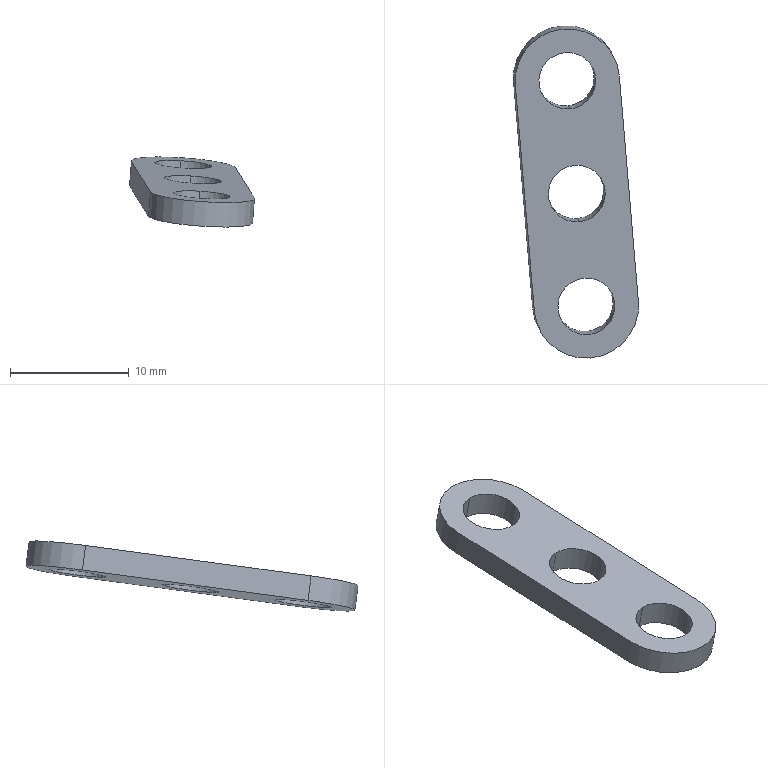Part | SolidWorks | features SplitBody 1 | 1 solid | 13 faces | box 10.521 x 27.955 x 5.897 mm | volume 365.029 mm3 | cylinder 9 | plane 4 | commonest cylinder face diameters 4.8 x6 8.8 x3
STEP:
#1=CARTESIAN_POINT('',(578.818,319.832,-356.747));
#2=VERTEX_POINT('',#1);
#3=CARTESIAN_POINT('',(579.217,315.091,-357.386));
#4=VERTEX_POINT('',#3);
#5=CARTESIAN_POINT('',(579.017,317.461,-357.067));
#6=DIRECTION('',(-0.07028,0.1275,-0.9893));
#7=DIRECTION('',(0.08315,-0.9876,-0.1332));
#8=AXIS2_PLACEMENT_3D('',#5,#6,#7);
#9=CIRCLE('',#8,2.4);
#10=EDGE_CURVE('',#2,#4,#9,.T.);
#11=ORIENTED_EDGE('',*,*,#10,.T.);
#12=CARTESIAN_POINT('',(579.363,314.826,-355.329));
#13=VERTEX_POINT('',#12);
#14=CARTESIAN_POINT('',(579.217,315.091,-357.386));
#15=DIRECTION('',(0.07028,-0.1275,0.9893));
#16=VECTOR('',#15,1000.);
#17=LINE('',#14,#16);
#18=EDGE_CURVE('',#4,#13,#17,.T.);
#19=ORIENTED_EDGE('',*,*,#18,.T.);
#20=CARTESIAN_POINT('',(578.964,319.566,-354.689));
#21=VERTEX_POINT('',#20);
#22=CARTESIAN_POINT('',(579.163,317.196,-355.009));
#23=DIRECTION('',(-0.07028,0.1275,-0.9893));
#24=DIRECTION('',(0.08315,-0.9876,-0.1332));
#25=AXIS2_PLACEMENT_3D('',#22,#23,#24);
#26=CIRCLE('',#25,2.4);
#27=EDGE_CURVE('',#21,#13,#26,.T.);
#28=ORIENTED_EDGE('',*,*,#27,.F.);
#29=CARTESIAN_POINT('',(578.818,319.832,-356.747));
#30=DIRECTION('',(0.07028,-0.1275,0.9893));
#31=VECTOR('',#30,1000.);
#32=LINE('',#29,#31);
#33=EDGE_CURVE('',#2,#21,#32,.T.);
#34=ORIENTED_EDGE('',*,*,#33,.F.);
#35=EDGE_LOOP('',(#11,#19,#28,#34));
#36=FACE_OUTER_BOUND('',#35,.T.);
#37=CARTESIAN_POINT('',(579.017,317.461,-357.067));
#38=DIRECTION('',(0.07028,-0.1275,0.9893));
#39=DIRECTION('',(-0.08315,0.9876,0.1332));
#40=AXIS2_PLACEMENT_3D('',#37,#38,#39);
#41=CYLINDRICAL_SURFACE('',#40,2.4);
#42=ADVANCED_FACE('',(#36),#41,.F.);
#43=CARTESIAN_POINT('',(578.019,329.312,-355.468));
#44=VERTEX_POINT('',#43);
#45=CARTESIAN_POINT('',(578.418,324.572,-356.108));
#46=VERTEX_POINT('',#45);
#47=CARTESIAN_POINT('',(578.219,326.942,-355.788));
#48=DIRECTION('',(-0.07028,0.1275,-0.9893));
#49=DIRECTION('',(0.08315,-0.9876,-0.1332));
#50=AXIS2_PLACEMENT_3D('',#47,#48,#49);
#51=CIRCLE('',#50,2.4);
#52=EDGE_CURVE('',#44,#46,#51,.T.);
#53=ORIENTED_EDGE('',*,*,#52,.T.);
#54=CARTESIAN_POINT('',(578.565,324.307,-354.05));
#55=VERTEX_POINT('',#54);
#56=CARTESIAN_POINT('',(578.418,324.572,-356.108));
#57=DIRECTION('',(0.07028,-0.1275,0.9893));
#58=VECTOR('',#57,1000.);
#59=LINE('',#56,#58);
#60=EDGE_CURVE('',#46,#55,#59,.T.);
#61=ORIENTED_EDGE('',*,*,#60,.T.);
#62=CARTESIAN_POINT('',(578.166,329.047,-353.411));
#63=VERTEX_POINT('',#62);
#64=CARTESIAN_POINT('',(578.365,326.677,-353.73));
#65=DIRECTION('',(-0.07028,0.1275,-0.9893));
#66=DIRECTION('',(0.08315,-0.9876,-0.1332));
#67=AXIS2_PLACEMENT_3D('',#64,#65,#66);
#68=CIRCLE('',#67,2.4);
#69=EDGE_CURVE('',#63,#55,#68,.T.);
#70=ORIENTED_EDGE('',*,*,#69,.F.);
#71=CARTESIAN_POINT('',(578.019,329.312,-355.468));
#72=DIRECTION('',(0.07028,-0.1275,0.9893));
#73=VECTOR('',#72,1000.);
#74=LINE('',#71,#73);
#75=EDGE_CURVE('',#44,#63,#74,.T.);
#76=ORIENTED_EDGE('',*,*,#75,.F.);
#77=EDGE_LOOP('',(#53,#61,#70,#76));
#78=FACE_OUTER_BOUND('',#77,.T.);
#79=CARTESIAN_POINT('',(578.219,326.942,-355.788));
#80=DIRECTION('',(0.07028,-0.1275,0.9893));
#81=DIRECTION('',(-0.08315,0.9876,0.1332));
#82=AXIS2_PLACEMENT_3D('',#79,#80,#81);
#83=CYLINDRICAL_SURFACE('',#82,2.4);
#84=ADVANCED_FACE('',(#78),#83,.F.);
#85=CARTESIAN_POINT('',(579.616,310.351,-358.026));
#86=VERTEX_POINT('',#85);
#87=CARTESIAN_POINT('',(580.015,305.61,-358.665));
#88=VERTEX_POINT('',#87);
#89=CARTESIAN_POINT('',(579.815,307.98,-358.345));
#90=DIRECTION('',(-0.07028,0.1275,-0.9893));
#91=DIRECTION('',(0.08315,-0.9876,-0.1332));
#92=AXIS2_PLACEMENT_3D('',#89,#90,#91);
#93=CIRCLE('',#92,2.4);
#94=EDGE_CURVE('',#86,#88,#93,.T.);
#95=ORIENTED_EDGE('',*,*,#94,.T.);
#96=CARTESIAN_POINT('',(580.161,305.345,-356.607));
#97=VERTEX_POINT('',#96);
#98=CARTESIAN_POINT('',(580.015,305.61,-358.665));
#99=DIRECTION('',(0.07028,-0.1275,0.9893));
#100=VECTOR('',#99,1000.);
#101=LINE('',#98,#100);
#102=EDGE_CURVE('',#88,#97,#101,.T.);
#103=ORIENTED_EDGE('',*,*,#102,.T.);
#104=CARTESIAN_POINT('',(579.762,310.085,-355.968));
#105=VERTEX_POINT('',#104);
#106=CARTESIAN_POINT('',(579.962,307.715,-356.288));
#107=DIRECTION('',(-0.07028,0.1275,-0.9893));
#108=DIRECTION('',(0.08315,-0.9876,-0.1332));
#109=AXIS2_PLACEMENT_3D('',#106,#107,#108);
#110=CIRCLE('',#109,2.4);
#111=EDGE_CURVE('',#105,#97,#110,.T.);
#112=ORIENTED_EDGE('',*,*,#111,.F.);
#113=CARTESIAN_POINT('',(579.616,310.351,-358.026));
#114=DIRECTION('',(0.07028,-0.1275,0.9893));
#115=VECTOR('',#114,1000.);
#116=LINE('',#113,#115);
#117=EDGE_CURVE('',#86,#105,#116,.T.);
#118=ORIENTED_EDGE('',*,*,#117,.F.);
#119=EDGE_LOOP('',(#95,#103,#112,#118));
#120=FACE_OUTER_BOUND('',#119,.T.);
#121=CARTESIAN_POINT('',(579.815,307.98,-358.345));
#122=DIRECTION('',(0.07028,-0.1275,0.9893));
#123=DIRECTION('',(-0.08315,0.9876,0.1332));
#124=AXIS2_PLACEMENT_3D('',#121,#122,#123);
#125=CYLINDRICAL_SURFACE('',#124,2.4);
#126=ADVANCED_FACE('',(#120),#125,.F.);
#127=CARTESIAN_POINT('',(577.853,331.288,-355.202));
#128=VERTEX_POINT('',#127);
#129=CARTESIAN_POINT('',(582.593,327.345,-356.047));
#130=VERTEX_POINT('',#129);
#131=CARTESIAN_POINT('',(578.219,326.942,-355.788));
#132=DIRECTION('',(-0.07028,0.1275,-0.9893));
#133=DIRECTION('',(-0.08315,0.9876,0.1332));
#134=AXIS2_PLACEMENT_3D('',#131,#132,#133);
#135=CIRCLE('',#134,4.4);
#136=EDGE_CURVE('',#128,#130,#135,.T.);
#137=ORIENTED_EDGE('',*,*,#136,.F.);
#138=CARTESIAN_POINT('',(577.999,331.022,-353.144));
#139=VERTEX_POINT('',#138);
#140=CARTESIAN_POINT('',(577.853,331.288,-355.202));
#141=DIRECTION('',(0.07028,-0.1275,0.9893));
#142=VECTOR('',#141,1000.);
#143=LINE('',#140,#142);
#144=EDGE_CURVE('',#128,#139,#143,.T.);
#145=ORIENTED_EDGE('',*,*,#144,.T.);
#146=CARTESIAN_POINT('',(582.739,327.08,-353.989));
#147=VERTEX_POINT('',#146);
#148=CARTESIAN_POINT('',(578.365,326.677,-353.73));
#149=DIRECTION('',(-0.07028,0.1275,-0.9893));
#150=DIRECTION('',(-0.08315,0.9876,0.1332));
#151=AXIS2_PLACEMENT_3D('',#148,#149,#150);
#152=CIRCLE('',#151,4.4);
#153=EDGE_CURVE('',#139,#147,#152,.T.);
#154=ORIENTED_EDGE('',*,*,#153,.T.);
#155=CARTESIAN_POINT('',(582.593,327.345,-356.047));
#156=DIRECTION('',(0.07028,-0.1275,0.9893));
#157=VECTOR('',#156,1000.);
#158=LINE('',#155,#157);
#159=EDGE_CURVE('',#130,#147,#158,.T.);
#160=ORIENTED_EDGE('',*,*,#159,.F.);
#161=EDGE_LOOP('',(#137,#145,#154,#160));
#162=FACE_OUTER_BOUND('',#161,.T.);
#163=CARTESIAN_POINT('',(578.219,326.942,-355.788));
#164=DIRECTION('',(0.07028,-0.1275,0.9893));
#165=DIRECTION('',(-0.08315,0.9876,0.1332));
#166=AXIS2_PLACEMENT_3D('',#163,#164,#165);
#167=CYLINDRICAL_SURFACE('',#166,4.4);
#168=ADVANCED_FACE('',(#162),#167,.T.);
#169=CARTESIAN_POINT('',(573.845,326.539,-355.529));
#170=VERTEX_POINT('',#169);
#171=CARTESIAN_POINT('',(578.219,326.942,-355.788));
#172=DIRECTION('',(-0.07028,0.1275,-0.9893));
#173=DIRECTION('',(-0.08315,0.9876,0.1332));
#174=AXIS2_PLACEMENT_3D('',#171,#172,#173);
#175=CIRCLE('',#174,4.4);
#176=EDGE_CURVE('',#170,#128,#175,.T.);
#177=ORIENTED_EDGE('',*,*,#176,.T.);
#178=ORIENTED_EDGE('',*,*,#136,.T.);
#179=CARTESIAN_POINT('',(584.189,308.384,-358.604));
#180=VERTEX_POINT('',#179);
#181=CARTESIAN_POINT('',(582.593,327.345,-356.047));
#182=DIRECTION('',(0.08315,-0.9876,-0.1332));
#183=VECTOR('',#182,1000.);
#184=LINE('',#181,#183);
#185=EDGE_CURVE('',#130,#180,#184,.T.);
#186=ORIENTED_EDGE('',*,*,#185,.T.);
#187=CARTESIAN_POINT('',(575.442,307.577,-358.087));
#188=VERTEX_POINT('',#187);
#189=CARTESIAN_POINT('',(579.815,307.98,-358.345));
#190=DIRECTION('',(-0.07028,0.1275,-0.9893));
#191=DIRECTION('',(0.08315,-0.9876,-0.1332));
#192=AXIS2_PLACEMENT_3D('',#189,#190,#191);
#193=CIRCLE('',#192,4.4);
#194=EDGE_CURVE('',#180,#188,#193,.T.);
#195=ORIENTED_EDGE('',*,*,#194,.T.);
#196=CARTESIAN_POINT('',(575.442,307.577,-358.087));
#197=DIRECTION('',(-0.08315,0.9876,0.1332));
#198=VECTOR('',#197,1000.);
#199=LINE('',#196,#198);
#200=EDGE_CURVE('',#188,#170,#199,.T.);
#201=ORIENTED_EDGE('',*,*,#200,.T.);
#202=EDGE_LOOP('',(#177,#178,#186,#195,#201));
#203=FACE_OUTER_BOUND('',#202,.T.);
#204=ORIENTED_EDGE('',*,*,#94,.F.);
#205=CARTESIAN_POINT('',(579.815,307.98,-358.345));
#206=DIRECTION('',(-0.07028,0.1275,-0.9893));
#207=DIRECTION('',(0.08315,-0.9876,-0.1332));
#208=AXIS2_PLACEMENT_3D('',#205,#206,#207);
#209=CIRCLE('',#208,2.4);
#210=EDGE_CURVE('',#88,#86,#209,.T.);
#211=ORIENTED_EDGE('',*,*,#210,.F.);
#212=EDGE_LOOP('',(#204,#211));
#213=FACE_BOUND('',#212,.T.);
#214=ORIENTED_EDGE('',*,*,#52,.F.);
#215=CARTESIAN_POINT('',(578.219,326.942,-355.788));
#216=DIRECTION('',(-0.07028,0.1275,-0.9893));
#217=DIRECTION('',(0.08315,-0.9876,-0.1332));
#218=AXIS2_PLACEMENT_3D('',#215,#216,#217);
#219=CIRCLE('',#218,2.4);
#220=EDGE_CURVE('',#46,#44,#219,.T.);
#221=ORIENTED_EDGE('',*,*,#220,.F.);
#222=EDGE_LOOP('',(#214,#221));
#223=FACE_BOUND('',#222,.T.);
#224=ORIENTED_EDGE('',*,*,#10,.F.);
#225=CARTESIAN_POINT('',(579.017,317.461,-357.067));
#226=DIRECTION('',(-0.07028,0.1275,-0.9893));
#227=DIRECTION('',(0.08315,-0.9876,-0.1332));
#228=AXIS2_PLACEMENT_3D('',#225,#226,#227);
#229=CIRCLE('',#228,2.4);
#230=EDGE_CURVE('',#4,#2,#229,.T.);
#231=ORIENTED_EDGE('',*,*,#230,.F.);
#232=EDGE_LOOP('',(#224,#231));
#233=FACE_BOUND('',#232,.T.);
#234=CARTESIAN_POINT('',(578.219,326.942,-355.788));
#235=DIRECTION('',(0.07028,-0.1275,0.9893));
#236=DIRECTION('',(-0.08315,0.9876,0.1332));
#237=AXIS2_PLACEMENT_3D('',#234,#235,#236);
#238=PLANE('',#237);
#239=ADVANCED_FACE('',(#203,#213,#223,#233),#238,.F.);
#240=ORIENTED_EDGE('',*,*,#69,.T.);
#241=CARTESIAN_POINT('',(578.365,326.677,-353.73));
#242=DIRECTION('',(-0.07028,0.1275,-0.9893));
#243=DIRECTION('',(0.08315,-0.9876,-0.1332));
#244=AXIS2_PLACEMENT_3D('',#241,#242,#243);
#245=CIRCLE('',#244,2.4);
#246=EDGE_CURVE('',#55,#63,#245,.T.);
#247=ORIENTED_EDGE('',*,*,#246,.T.);
#248=EDGE_LOOP('',(#240,#247));
#249=FACE_BOUND('',#248,.T.);
#250=CARTESIAN_POINT('',(573.991,326.274,-353.471));
#251=VERTEX_POINT('',#250);
#252=CARTESIAN_POINT('',(578.365,326.677,-353.73));
#253=DIRECTION('',(-0.07028,0.1275,-0.9893));
#254=DIRECTION('',(-0.08315,0.9876,0.1332));
#255=AXIS2_PLACEMENT_3D('',#252,#253,#254);
#256=CIRCLE('',#255,4.4);
#257=EDGE_CURVE('',#251,#139,#256,.T.);
#258=ORIENTED_EDGE('',*,*,#257,.F.);
#259=CARTESIAN_POINT('',(575.588,307.312,-356.029));
#260=VERTEX_POINT('',#259);
#261=CARTESIAN_POINT('',(575.588,307.312,-356.029));
#262=DIRECTION('',(-0.08315,0.9876,0.1332));
#263=VECTOR('',#262,1000.);
#264=LINE('',#261,#263);
#265=EDGE_CURVE('',#260,#251,#264,.T.);
#266=ORIENTED_EDGE('',*,*,#265,.F.);
#267=CARTESIAN_POINT('',(584.335,308.118,-356.546));
#268=VERTEX_POINT('',#267);
#269=CARTESIAN_POINT('',(579.962,307.715,-356.288));
#270=DIRECTION('',(-0.07028,0.1275,-0.9893));
#271=DIRECTION('',(0.08315,-0.9876,-0.1332));
#272=AXIS2_PLACEMENT_3D('',#269,#270,#271);
#273=CIRCLE('',#272,4.4);
#274=EDGE_CURVE('',#268,#260,#273,.T.);
#275=ORIENTED_EDGE('',*,*,#274,.F.);
#276=CARTESIAN_POINT('',(582.739,327.08,-353.989));
#277=DIRECTION('',(0.08315,-0.9876,-0.1332));
#278=VECTOR('',#277,1000.);
#279=LINE('',#276,#278);
#280=EDGE_CURVE('',#147,#268,#279,.T.);
#281=ORIENTED_EDGE('',*,*,#280,.F.);
#282=ORIENTED_EDGE('',*,*,#153,.F.);
#283=EDGE_LOOP('',(#258,#266,#275,#281,#282));
#284=FACE_OUTER_BOUND('',#283,.T.);
#285=ORIENTED_EDGE('',*,*,#111,.T.);
#286=CARTESIAN_POINT('',(579.962,307.715,-356.288));
#287=DIRECTION('',(-0.07028,0.1275,-0.9893));
#288=DIRECTION('',(0.08315,-0.9876,-0.1332));
#289=AXIS2_PLACEMENT_3D('',#286,#287,#288);
#290=CIRCLE('',#289,2.4);
#291=EDGE_CURVE('',#97,#105,#290,.T.);
#292=ORIENTED_EDGE('',*,*,#291,.T.);
#293=EDGE_LOOP('',(#285,#292));
#294=FACE_BOUND('',#293,.T.);
#295=ORIENTED_EDGE('',*,*,#27,.T.);
#296=CARTESIAN_POINT('',(579.163,317.196,-355.009));
#297=DIRECTION('',(-0.07028,0.1275,-0.9893));
#298=DIRECTION('',(0.08315,-0.9876,-0.1332));
#299=AXIS2_PLACEMENT_3D('',#296,#297,#298);
#300=CIRCLE('',#299,2.4);
#301=EDGE_CURVE('',#13,#21,#300,.T.);
#302=ORIENTED_EDGE('',*,*,#301,.T.);
#303=EDGE_LOOP('',(#295,#302));
#304=FACE_BOUND('',#303,.T.);
#305=CARTESIAN_POINT('',(578.365,326.677,-353.73));
#306=DIRECTION('',(0.07028,-0.1275,0.9893));
#307=DIRECTION('',(-0.08315,0.9876,0.1332));
#308=AXIS2_PLACEMENT_3D('',#305,#306,#307);
#309=PLANE('',#308);
#310=ADVANCED_FACE('',(#249,#284,#294,#304),#309,.T.);
#311=ORIENTED_EDGE('',*,*,#144,.F.);
#312=ORIENTED_EDGE('',*,*,#176,.F.);
#313=CARTESIAN_POINT('',(573.845,326.539,-355.529));
#314=DIRECTION('',(0.07028,-0.1275,0.9893));
#315=VECTOR('',#314,1000.);
#316=LINE('',#313,#315);
#317=EDGE_CURVE('',#170,#251,#316,.T.);
#318=ORIENTED_EDGE('',*,*,#317,.T.);
#319=ORIENTED_EDGE('',*,*,#257,.T.);
#320=EDGE_LOOP('',(#311,#312,#318,#319));
#321=FACE_OUTER_BOUND('',#320,.T.);
#322=CARTESIAN_POINT('',(578.219,326.942,-355.788));
#323=DIRECTION('',(0.07028,-0.1275,0.9893));
#324=DIRECTION('',(-0.08315,0.9876,0.1332));
#325=AXIS2_PLACEMENT_3D('',#322,#323,#324);
#326=CYLINDRICAL_SURFACE('',#325,4.4);
#327=ADVANCED_FACE('',(#321),#326,.T.);
#328=ORIENTED_EDGE('',*,*,#280,.T.);
#329=CARTESIAN_POINT('',(584.189,308.384,-358.604));
#330=DIRECTION('',(0.07028,-0.1275,0.9893));
#331=VECTOR('',#330,1000.);
#332=LINE('',#329,#331);
#333=EDGE_CURVE('',#180,#268,#332,.T.);
#334=ORIENTED_EDGE('',*,*,#333,.F.);
#335=ORIENTED_EDGE('',*,*,#185,.F.);
#336=ORIENTED_EDGE('',*,*,#159,.T.);
#337=EDGE_LOOP('',(#328,#334,#335,#336));
#338=FACE_OUTER_BOUND('',#337,.T.);
#339=CARTESIAN_POINT('',(582.593,327.345,-356.047));
#340=DIRECTION('',(-0.9941,-0.09163,0.0588));
#341=DIRECTION('',(-0.08315,0.9876,0.1332));
#342=AXIS2_PLACEMENT_3D('',#339,#340,#341);
#343=PLANE('',#342);
#344=ADVANCED_FACE('',(#338),#343,.F.);
#345=ORIENTED_EDGE('',*,*,#274,.T.);
#346=CARTESIAN_POINT('',(575.442,307.577,-358.087));
#347=DIRECTION('',(0.07028,-0.1275,0.9893));
#348=VECTOR('',#347,1000.);
#349=LINE('',#346,#348);
#350=EDGE_CURVE('',#188,#260,#349,.T.);
#351=ORIENTED_EDGE('',*,*,#350,.F.);
#352=ORIENTED_EDGE('',*,*,#194,.F.);
#353=ORIENTED_EDGE('',*,*,#333,.T.);
#354=EDGE_LOOP('',(#345,#351,#352,#353));
#355=FACE_OUTER_BOUND('',#354,.T.);
#356=CARTESIAN_POINT('',(579.815,307.98,-358.345));
#357=DIRECTION('',(0.07028,-0.1275,0.9893));
#358=DIRECTION('',(-0.08315,0.9876,0.1332));
#359=AXIS2_PLACEMENT_3D('',#356,#357,#358);
#360=CYLINDRICAL_SURFACE('',#359,4.4);
#361=ADVANCED_FACE('',(#355),#360,.T.);
#362=ORIENTED_EDGE('',*,*,#265,.T.);
#363=ORIENTED_EDGE('',*,*,#317,.F.);
#364=ORIENTED_EDGE('',*,*,#200,.F.);
#365=ORIENTED_EDGE('',*,*,#350,.T.);
#366=EDGE_LOOP('',(#362,#363,#364,#365));
#367=FACE_OUTER_BOUND('',#366,.T.);
#368=CARTESIAN_POINT('',(575.442,307.577,-358.087));
#369=DIRECTION('',(0.9941,0.09163,-0.0588));
#370=DIRECTION('',(0.08315,-0.9876,-0.1332));
#371=AXIS2_PLACEMENT_3D('',#368,#369,#370);
#372=PLANE('',#371);
#373=ADVANCED_FACE('',(#367),#372,.F.);
#374=ORIENTED_EDGE('',*,*,#102,.F.);
#375=ORIENTED_EDGE('',*,*,#210,.T.);
#376=ORIENTED_EDGE('',*,*,#117,.T.);
#377=ORIENTED_EDGE('',*,*,#291,.F.);
#378=EDGE_LOOP('',(#374,#375,#376,#377));
#379=FACE_OUTER_BOUND('',#378,.T.);
#380=CARTESIAN_POINT('',(579.815,307.98,-358.345));
#381=DIRECTION('',(0.07028,-0.1275,0.9893));
#382=DIRECTION('',(-0.08315,0.9876,0.1332));
#383=AXIS2_PLACEMENT_3D('',#380,#381,#382);
#384=CYLINDRICAL_SURFACE('',#383,2.4);
#385=ADVANCED_FACE('',(#379),#384,.F.);
#386=ORIENTED_EDGE('',*,*,#60,.F.);
#387=ORIENTED_EDGE('',*,*,#220,.T.);
#388=ORIENTED_EDGE('',*,*,#75,.T.);
#389=ORIENTED_EDGE('',*,*,#246,.F.);
#390=EDGE_LOOP('',(#386,#387,#388,#389));
#391=FACE_OUTER_BOUND('',#390,.T.);
#392=CARTESIAN_POINT('',(578.219,326.942,-355.788));
#393=DIRECTION('',(0.07028,-0.1275,0.9893));
#394=DIRECTION('',(-0.08315,0.9876,0.1332));
#395=AXIS2_PLACEMENT_3D('',#392,#393,#394);
#396=CYLINDRICAL_SURFACE('',#395,2.4);
#397=ADVANCED_FACE('',(#391),#396,.F.);
#398=ORIENTED_EDGE('',*,*,#18,.F.);
#399=ORIENTED_EDGE('',*,*,#230,.T.);
#400=ORIENTED_EDGE('',*,*,#33,.T.);
#401=ORIENTED_EDGE('',*,*,#301,.F.);
#402=EDGE_LOOP('',(#398,#399,#400,#401));
#403=FACE_OUTER_BOUND('',#402,.T.);
#404=CARTESIAN_POINT('',(579.017,317.461,-357.067));
#405=DIRECTION('',(0.07028,-0.1275,0.9893));
#406=DIRECTION('',(-0.08315,0.9876,0.1332));
#407=AXIS2_PLACEMENT_3D('',#404,#405,#406);
#408=CYLINDRICAL_SURFACE('',#407,2.4);
#409=ADVANCED_FACE('',(#403),#408,.F.);
#410=CLOSED_SHELL('',(#42,#84,#126,#168,#239,#310,#327,#344,#361,#373,#385,#397,#409));
#411=MANIFOLD_SOLID_BREP('',#410);
#412=CARTESIAN_POINT('',(0.,0.,0.));
#413=DIRECTION('',(0.,0.,1.));
#414=DIRECTION('',(1.,0.,0.));
#415=AXIS2_PLACEMENT_3D('',#412,#413,#414);
#416=(LENGTH_UNIT()NAMED_UNIT(*)SI_UNIT(.MILLI.,.METRE.));
#417=UNCERTAINTY_MEASURE_WITH_UNIT(LENGTH_MEASURE(0.00001),#416,'','');
#418=(NAMED_UNIT(*)PLANE_ANGLE_UNIT()SI_UNIT($,.RADIAN.));
#419=(NAMED_UNIT(*)SI_UNIT($,.STERADIAN.)SOLID_ANGLE_UNIT());
#420=(GEOMETRIC_REPRESENTATION_CONTEXT(3)GLOBAL_UNCERTAINTY_ASSIGNED_CONTEXT((#417))GLOBAL_UNIT_ASSIGNED_CONTEXT((#416,#418,#419))REPRESENTATION_CONTEXT('',''));
#421=ADVANCED_BREP_SHAPE_REPRESENTATION('',(#411,#415),#420);